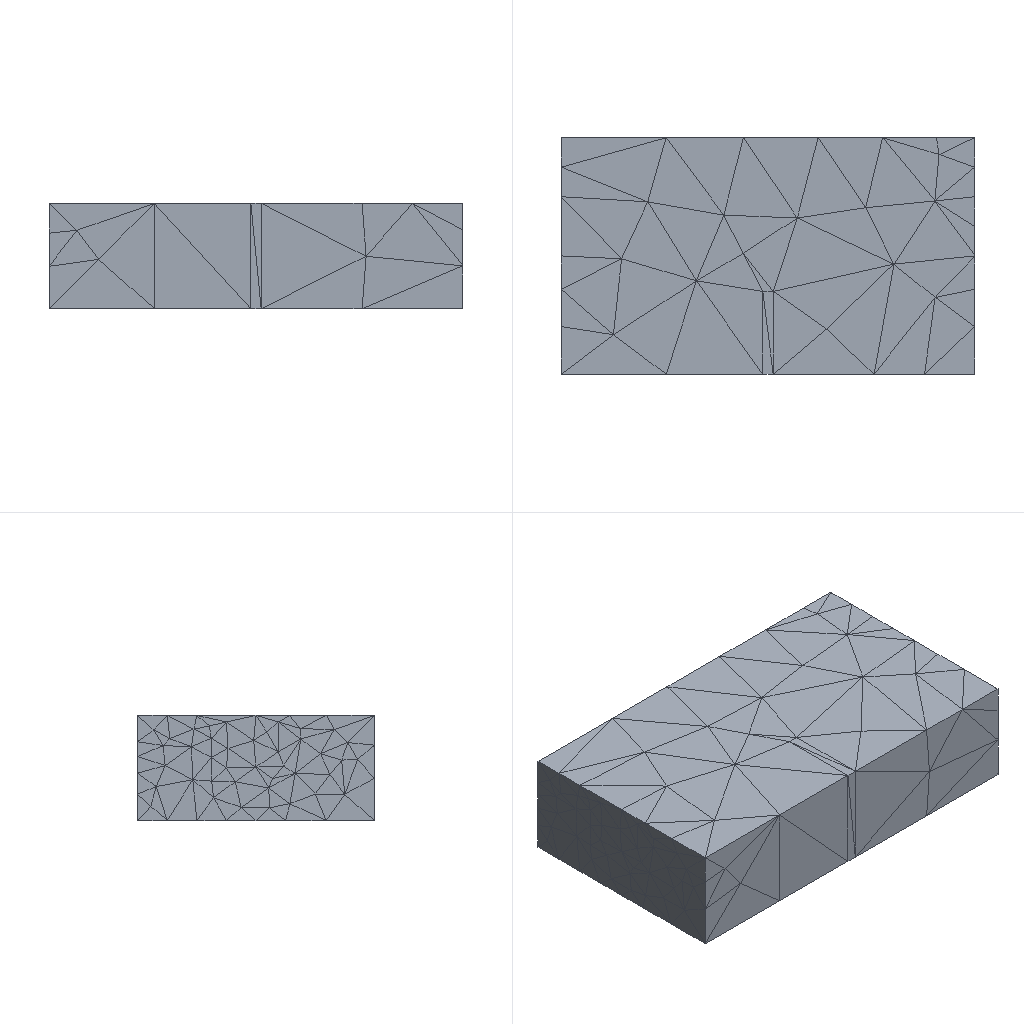Simulation study | ansys electronics desktop
Set-up summary:
category,name,step,type,value,unit,region
solver,ansys_electronics_desktop
units,length mm,,stated,model units
analysis,M16,,HFSS Modal Network,design_type=HFSS
setup,Setup1,M16,HfssDriven,frequency=10GHz; max_passes=2; max_delta_s=0.08
sweep,Sweep1,Setup1,Interpolating,8GHz..12GHz n=11 step=
mesh,nodes,,,n/a (no mesh stored)
mesh,elements,,,n/a (no mesh stored)
material,vacuum,,permittivity,1
load,P1,M16,wave port,,,objects 62
load,P2,M16,wave port,,,objects 74
bc,PerfE_VVAXO5,M16,perfect e,,,objects 86
bc,PerfE_TDHT5O,M16,perfect e,,,objects 98
bc,PerfE_5OTQQF,M16,perfect e,,,objects 110
bc,PerfE_AXHEQ4,M16,perfect e,,,objects 122
Ansys Electronics Desktop project file, long lists of numbers shortened, first 681 of 3558 lines:
$begin 'AnsoftProject'
	Created='Wed Sep 30 18:16:44 2026'
	Product='ElectronicsDesktop'
	FileOwnedByWorkbench=false
	$begin 'Desktop'
		Version(2026, 1)
		InfrastructureVersion(1, 0)
		$begin 'FactoryHeader'
			$begin 'geometry3deditor'
				KernelVersion(2, 0)
				ProjectContainsGeometry3D='1'
			$end 'geometry3deditor'
		$end 'FactoryHeader'
	$end 'Desktop'
	UsesAdvancedFeatures=false
	PreviewImageDesignId=1
	NextUniqueID=0
	MoveBackwards=false
	$begin 'HFSSEnvironment'
		Version(1, 0)
	$end 'HFSSEnvironment'
	$begin 'PlanarEMEnvironment'
		Version(1, 0)
	$end 'PlanarEMEnvironment'
	$begin 'Q3DEnvironment'
		Version(1, 0)
	$end 'Q3DEnvironment'
	$begin '2DExtractorEnvironment'
		Version(1, 0)
	$end '2DExtractorEnvironment'
	$begin 'NexximEnvironment'
		Version(1, 0)
	$end 'NexximEnvironment'
	$begin 'NexximNetlistEnvironment'
		Version(1, 0)
	$end 'NexximNetlistEnvironment'
	$begin 'EmitEnvironment'
		Version(1, 0)
	$end 'EmitEnvironment'
	$begin 'Maxwell3DEnvironment'
		Version(1, 0)
	$end 'Maxwell3DEnvironment'
	$begin 'Maxwell2DEnvironment'
		Version(1, 0)
	$end 'Maxwell2DEnvironment'
	$begin 'RMxprtEnvironment'
		Version(1, 0)
	$end 'RMxprtEnvironment'
	$begin 'MaxCirEnvironment'
		Version(1, 0)
	$end 'MaxCirEnvironment'
	$begin 'SimplorerEnvironment'
		Version(1, 0)
	$end 'SimplorerEnvironment'
	$begin 'IcepakEnvironment'
		Version(1, 0)
	$end 'IcepakEnvironment'
	$begin 'IcepakFEAEnvironment'
		Version(1, 0)
	$end 'IcepakFEAEnvironment'
	$begin 'SchematicEnvironment'
		Version(1, 0)
	$end 'SchematicEnvironment'
	$begin 'geometry3deditor'
		Version(1, 0)
	$end 'geometry3deditor'
	ReadVersion=12
	$begin 'DesignMgrEnvironment'
		CompInstCounter=1
		GPortCounter=0
		NetCounter=0
		Alias('Ieee;Simplorer Elements\\Ieee', 'Std;Simplorer Elements\\Std', 'Basic_VHDLAMS;Simplorer Elements\\Basic Elements VHDLAMS\\Basic Elements VHDLAMS', 'Digital_Elements;Simplorer Elements\\Digital Elements\\Digital Elements', 'Transformations;Simplorer Elements\\Tools\\Transformations\\Transformations', 'HEV_VHDLAMS;Simplorer Elements\\HEV VHDLAMS\\HEV VHDLAMS', 'automotive_vda;Simplorer Elem
	$end 'DesignMgrEnvironment'
	$begin 'ProjectDatasets'
		NextUniqueID=0
		MoveBackwards=false
		DatasetType='ProjectDatasetType'
		$begin 'DatasetDefinitions'
		$end 'DatasetDefinitions'
	$end 'ProjectDatasets'
	VariableOrders[0:]
	$begin 'Definitions'
		$begin 'Materials'
			$begin 'vacuum'
				CoordinateSystemType='Cartesian'
				BulkOrSurfaceType=1
				$begin 'PhysicsTypes'
					set('Electromagnetic')
				$end 'PhysicsTypes'
				$begin 'AttachedData'
					$begin 'MatAppearanceData'
						property_data='appearance_data'
						Red=230
						Green=230
						Blue=230
						Transparency=0.95
					$end 'MatAppearanceData'
				$end 'AttachedData'
				permittivity='1'
				ModTime=1499970477
				Library='Materials'
				LibLocation='SysLibrary'
				ModSinceLib=false
			$end 'vacuum'
		$end 'Materials'
		$begin 'SurfaceMaterials'
		$end 'SurfaceMaterials'
		$begin 'Scripts'
		$end 'Scripts'
		$begin 'AnsysComponents'
			NextUniqueID=0
			MoveBackwards=false
			$begin 'AnsysComponentDefinitions'
			$end 'AnsysComponentDefinitions'
		$end 'AnsysComponents'
		$begin 'Symbols'
			$begin 'M16'
				ModTime=1790763405
				Library=''
				ModSinceLib=false
				LibLocation='Project'
				HighestLevel=1
				Normalize=true
				InitialLevels(0, 1)
				$begin 'Graphics'
					Rect(0, 0, 0, 0, 0.00254, 0.00254, 0.00508, 0.00508, 0, 0, 0)
					Rect(0, 1, 0, 0, 0.0004233, 0.00254, 0.0004233, 0.0004233, 0, 0, 0)
				$end 'Graphics'
			$end 'M16'
		$end 'Symbols'
		$begin 'DefInfo'
			M16(1002, 0, 0, 0, '', 1790763405, '', 'M16', '', '', '', '', '', 'Design.bmp', '', 'Project', '', '', 1790763405, '', 0, 0)
		$end 'DefInfo'
		$begin 'Compdefs'
			$begin 'M16'
				Library=''
				CircuitEnv=0
				Refbase='U'
				NumParts=1
				ModSinceLib=true
				$begin 'Properties'
					TextProp('Representation', 'SRD', '', 'M16')
					TextProp('Owner', 'SRD', '', 'HFSS')
				$end 'Properties'
				CompExtID=6
				$begin 'Parameters'
					ButtonProp('CosimDefinition', 'D', '', 'Edit', 'Edit', 40501, ButtonPropClientData())
					MenuProp('CoSimulator', 'D', '', 'DefaultNetlist', 0)
				$end 'Parameters'
				$begin 'CosimDefinitions'
					$begin 'CosimDefinition'
						CosimulatorType=4
						CosimDefName='DefaultNetlist'
						IsDefinition=true
						Connect=true
						Data()
						GRef()
					$end 'CosimDefinition'
					DefaultCosim='DefaultNetlist'
				$end 'CosimDefinitions'
			$end 'M16'
		$end 'Compdefs'
	$end 'Definitions'
	DesignIDServer=2
	MoveBackwards=false
	$begin 'HFSSModel'
		RepRewriteV2=true
		Name='M16'
		DesignID=0
		'Use Advanced DC Extrapolation'=false
		'Use Power S'=false
		'Export FRTM After Simulation'=false
		'Export Rays After Simulation'=false
		'Export After Simulation'=false
		'Allow Material Override'=false
		'Calculate Lossy Dielectrics'=false
		'Perform Minimal validation'=false
		$begin 'TemperatureSettings'
			IncludeTemperatureDependence=false
			EnableFeedback=false
			Temperatures(6, '22cel', 34, '22cel', 62, '22cel', 74, '22cel', 86, '22cel', 98, '22cel', 110, '22cel', 122, '22cel')
		$end 'TemperatureSettings'
		ObjsEnabledForDeformation()
		'Port Validation Settings'='Standard'
		'Save Adaptive support files'=false
		SolutionType='HFSS Modal Network'
		$begin 'DrivenOptions'
			AutoOpen=false
		$end 'DrivenOptions'
		HasTransientSetups=false
		MaterialDensity=1
		MassOfTissue=1
		VoxelSize=1
		TissueObjectList=-1
		AverageSarMethod=0
		UseAutoDCThickness=true
		HaveZwaveSupport=true
		SolveInsideThreshold=100000
		RequireBodyFaceInfo=false
		$begin 'OutputVariable'
			NextUniqueID=0
			MoveBackwards=false
		$end 'OutputVariable'
		$begin 'ModelSetup'
			$begin 'DesignDatasets'
				NextUniqueID=0
				MoveBackwards=false
				DatasetType='DesignDatasetType'
				$begin 'DatasetDefinitions'
				$end 'DatasetDefinitions'
			$end 'DesignDatasets'
			VariableOrders[0:]
			$begin 'Editor3D Doc Preferences'
				BackgroundColorVersion=1
				'Plane Background'=0
				'Need Lights'=true
				'Ambient Light'=8355711
				'Num Lights'=1
				Light0[4: 16777215, 0.75, -0.15, -0.63]
				Ver=2
			$end 'Editor3D Doc Preferences'
			SnapMode=31
			WorkingCS=1
			$begin 'GeometryCore'
				BlockVersionID=3
				DataVersion=2
				NativeKernel='PARASOLID'
				NativeKernelVersionID=26
				Units='mm'
				ModelExtents=10000
				InstanceID=-1
				$begin 'ValidationOptions'
					EntityCheckLevel='Strict'
					IgnoreUnclassifiedObjects=false
					SkipIntersectionChecks=false
				$end 'ValidationOptions'
				ContainsGeomLinkUDM=false
				$begin 'GeometryOperations'
					BlockVersionID=2
					$begin 'AnsoftRangedIDServerManager'
						$begin 'AnsoftRangedIDServer'
							IDServerObjectTypeID=0
							IDServerRangeMin=0
							IDServerRangeMax=2146483647
							NextUniqueID=133
							MoveBackwards=false
						$end 'AnsoftRangedIDServer'
						$begin 'AnsoftRangedIDServer'
							IDServerObjectTypeID=1
							IDServerRangeMin=2146483648
							IDServerRangeMax=2146485547
							NextUniqueID=2146483654
							MoveBackwards=false
						$end 'AnsoftRangedIDServer'
					$end 'AnsoftRangedIDServerManager'
					StartBackGroundFaceID=2146483648
					$begin 'CoordinateSystems'
					$end 'CoordinateSystems'
					$begin 'OperandCSs'
					$end 'OperandCSs'
					$begin 'SubModelDefinitions'
					$end 'SubModelDefinitions'
					$begin 'Groups'
					$end 'Groups'
					$begin 'UserDefinedModels'
					$end 'UserDefinedModels'
					$begin 'OperandUserDefinedModels'
					$end 'OperandUserDefinedModels'
					$begin 'ToplevelParts'
						$begin 'GeometryPart'
							$begin 'Attributes'
								Name='WG'
								Flags=''
								Color='(230 230 230)'
								Transparency=0.8
								PartCoordinateSystem=1
								UDMId=-1
								GroupId=-1
								MaterialValue='"vacuum"'
								SurfaceMaterialValue='""'
								SolveInside=true
								ShellElement=false
								ShellElementThickness='0mm'
								ReferenceTemperature='20cel'
								IsMaterialEditable=true
								IsSurfaceMaterialEditable=true
								UseMaterialAppearance=false
								IsLightweight=false
								IsAlwaysHidden=false
							$end 'Attributes'
							$begin 'PhysicsAttributes'
								SuppressedForPhysics='False'
								SuppressedForPhysicsEditable=true
							$end 'PhysicsAttributes'
							$begin 'Operations'
								$begin 'Operation'
									OperationType='Box'
									ID=5
									ReferenceCoordSystemID=1
									$begin 'BoxParameters'
										KernelVersion=23
										XPosition='0mm'
										YPosition='0mm'
										ZPosition='0mm'
										XSize='40mm'
										YSize='22.86mm'
										ZSize='10.16mm'
									$end 'BoxParameters'
									ParentPartID=6
									ReferenceUDMID=-1
									IsSuppressed=false
									$begin 'OperationIdentity'
										$begin 'Topology'
											NumLumps=1
											NumShells=1
											NumFaces=6
											NumWires=0
											NumLoops=6
											NumCoedges=24
											NumEdges=12
											NumVertices=8
										$end 'Topology'
										BodyID=6
										StartFaceID=7
										StartEdgeID=13
										StartVertexID=25
										NumNewFaces=6
										NumNewEdges=12
										NumNewVertices=8
										FaceNameAndIDMap()
										EdgeNameAndIDMap()
										VertexNameAndIDMap()
									$end 'OperationIdentity'
								$end 'Operation'
							$end 'Operations'
							$begin 'SubregionDependencyInformation'
								ChildSubregions[0:]
							$end 'SubregionDependencyInformation'
						$end 'GeometryPart'
						$begin 'GeometryPart'
							$begin 'Attributes'
								Name='Iris'
								Flags=''
								Color='(230 230 230)'
								Transparency=0.8
								PartCoordinateSystem=1
								UDMId=-1
								GroupId=-1
								MaterialValue='"vacuum"'
								SurfaceMaterialValue='""'
								SolveInside=true
								ShellElement=false
								ShellElementThickness='0mm'
								ReferenceTemperature='20cel'
								IsMaterialEditable=true
								IsSurfaceMaterialEditable=true
								UseMaterialAppearance=false
								IsLightweight=false
								IsAlwaysHidden=false
							$end 'Attributes'
							$begin 'PhysicsAttributes'
								SuppressedForPhysics='False'
								SuppressedForPhysicsEditable=true
							$end 'PhysicsAttributes'
							$begin 'Operations'
								$begin 'Operation'
									OperationType='Box'
									ID=33
									ReferenceCoordSystemID=1
									$begin 'BoxParameters'
										KernelVersion=23
										XPosition='19.5mm'
										YPosition='0mm'
										ZPosition='0mm'
										XSize='1mm'
										YSize='8.001mm'
										ZSize='10.16mm'
									$end 'BoxParameters'
									ParentPartID=34
									ReferenceUDMID=-1
									IsSuppressed=false
									$begin 'OperationIdentity'
										$begin 'Topology'
											NumLumps=1
											NumShells=1
											NumFaces=6
											NumWires=0
											NumLoops=6
											NumCoedges=24
											NumEdges=12
											NumVertices=8
										$end 'Topology'
										BodyID=34
										StartFaceID=35
										StartEdgeID=41
										StartVertexID=53
										NumNewFaces=6
										NumNewEdges=12
										NumNewVertices=8
										FaceNameAndIDMap()
										EdgeNameAndIDMap()
										VertexNameAndIDMap()
									$end 'OperationIdentity'
								$end 'Operation'
							$end 'Operations'
							$begin 'SubregionDependencyInformation'
								ChildSubregions[0:]
							$end 'SubregionDependencyInformation'
						$end 'GeometryPart'
						$begin 'GeometryPart'
							$begin 'Attributes'
								Name='Port1'
								Flags=''
								Color='(230 230 230)'
								Transparency=0.8
								PartCoordinateSystem=1
								UDMId=-1
								GroupId=-1
								MaterialValue='"vacuum"'
								SurfaceMaterialValue='""'
								SolveInside=true
								ShellElement=false
								ShellElementThickness='0mm'
								ReferenceTemperature='20cel'
								IsMaterialEditable=true
								IsSurfaceMaterialEditable=true
								UseMaterialAppearance=false
								IsLightweight=false
								IsAlwaysHidden=false
							$end 'Attributes'
							$begin 'PhysicsAttributes'
								SuppressedForPhysics='False'
								SuppressedForPhysicsEditable=true
							$end 'PhysicsAttributes'
							$begin 'Operations'
								$begin 'Operation'
									OperationType='Rectangle'
									ID=61
									ReferenceCoordSystemID=1
									$begin 'RectangleParameters'
										KernelVersion=23
										XStart='0mm'
										YStart='0mm'
										ZStart='0mm'
										Width='22.86mm'
										Height='10.16mm'
										WhichAxis='X'
									$end 'RectangleParameters'
									ParentPartID=62
									ReferenceUDMID=-1
									IsSuppressed=false
									$begin 'OperationIdentity'
										$begin 'Topology'
											NumLumps=1
											NumShells=1
											NumFaces=0
											NumWires=1
											NumLoops=0
											NumCoedges=0
											NumEdges=4
											NumVertices=4
										$end 'Topology'
										BodyID=62
										StartFaceID=-1
										StartEdgeID=63
										StartVertexID=67
										NumNewFaces=0
										NumNewEdges=4
										NumNewVertices=4
										FaceNameAndIDMap()
										EdgeNameAndIDMap()
										VertexNameAndIDMap()
									$end 'OperationIdentity'
								$end 'Operation'
								$begin 'Operation'
									OperationType='CoverLines'
									ID=71
									$begin 'LocalOperationParameters'
										KernelVersion=23
										LocalOpPart=62
									$end 'LocalOperationParameters'
									ParentPartID=62
									ReferenceUDMID=-1
									IsSuppressed=false
									$begin 'OperationIdentity'
										$begin 'Topology'
											NumLumps=1
											NumShells=1
											NumFaces=1
											NumWires=0
											NumLoops=1
											NumCoedges=4
											NumEdges=4
											NumVertices=4
										$end 'Topology'
										BodyID=-1
										StartFaceID=72
										StartEdgeID=-1
										StartVertexID=-1
										NumNewFaces=1
										NumNewEdges=0
										NumNewVertices=0
										FaceNameAndIDMap()
										EdgeNameAndIDMap()
										VertexNameAndIDMap()
										$begin 'GeomTopolBasedOperationIdentityHelper'
											$begin 'NewFaces'
												$begin 'Face'
													NormalizedSerialNum=0
													ID=72
													$begin 'FaceGeomTopol'
														FaceTopol(1, 4, 4, 4)
														$begin 'FaceGeometry'
															Area=232.258
															FcUVMid(1.51681195174844e-15, 11.43, 5.08)
															$begin 'FcTolVts'
																TolVt(0, 0, 0, 5e-07)
																TolVt(1.39977129142543e-15, 22.86, 5.07593966858622e-15, 5e-07)
																TolVt(3.03362390349689e-15, 22.86, 10.16, 5e-07)
																TolVt(1.63385261207146e-15, -2.25597318603832e-15, 10.16, 5e-07)
															$end 'FcTolVts'
														$end 'FaceGeometry'
													$end 'FaceGeomTopol'
												$end 'Face'
											$end 'NewFaces'
											$begin 'NewEdges'
											$end 'NewEdges'
											$begin 'NewVertices'
											$end 'NewVertices'
										$end 'GeomTopolBasedOperationIdentityHelper'
									$end 'OperationIdentity'
									ParentOperationID=61
								$end 'Operation'
							$end 'Operations'
							$begin 'SubregionDependencyInformation'
								ChildSubregions[0:]
							$end 'SubregionDependencyInformation'
						$end 'GeometryPart'
						$begin 'GeometryPart'
							$begin 'Attributes'
								Name='Port2'
								Flags=''
								Color='(230 230 230)'
								Transparency=0.8
								PartCoordinateSystem=1
								UDMId=-1
								GroupId=-1
								MaterialValue='"vacuum"'
								SurfaceMaterialValue='""'
								SolveInside=true
								ShellElement=false
								ShellElementThickness='0mm'
								ReferenceTemperature='20cel'
								IsMaterialEditable=true
								IsSurfaceMaterialEditable=true
								UseMaterialAppearance=false
								IsLightweight=false
								IsAlwaysHidden=false
							$end 'Attributes'
							$begin 'PhysicsAttributes'
								SuppressedForPhysics='False'
								SuppressedForPhysicsEditable=true
							$end 'PhysicsAttributes'
							$begin 'Operations'
								$begin 'Operation'
									OperationType='Rectangle'
									ID=73
									ReferenceCoordSystemID=1
									$begin 'RectangleParameters'
										KernelVersion=23
										XStart='40mm'
										YStart='0mm'
										ZStart='0mm'
										Width='22.86mm'
										Height='10.16mm'
										WhichAxis='X'
									$end 'RectangleParameters'
									ParentPartID=74
									ReferenceUDMID=-1
									IsSuppressed=false
									$begin 'OperationIdentity'
										$begin 'Topology'
											NumLumps=1
											NumShells=1
											NumFaces=0
											NumWires=1
											NumLoops=0
											NumCoedges=0
											NumEdges=4
											NumVertices=4
										$end 'Topology'
										BodyID=74
										StartFaceID=-1
										StartEdgeID=75
										StartVertexID=79
										NumNewFaces=0
										NumNewEdges=4
										NumNewVertices=4
										FaceNameAndIDMap()
										EdgeNameAndIDMap()
										VertexNameAndIDMap()
									$end 'OperationIdentity'
								$end 'Operation'
								$begin 'Operation'
									OperationType='CoverLines'
									ID=83
									$begin 'LocalOperationParameters'
										KernelVersion=23
										LocalOpPart=74
									$end 'LocalOperationParameters'
									ParentPartID=74
									ReferenceUDMID=-1
									IsSuppressed=false
									$begin 'OperationIdentity'
										$begin 'Topology'
											NumLumps=1
											NumShells=1
											NumFaces=1
											NumWires=0
											NumLoops=1
											NumCoedges=4
											NumEdges=4
											NumVertices=4
										$end 'Topology'
										BodyID=-1
										StartFaceID=84
										StartEdgeID=-1
										StartVertexID=-1
										NumNewFaces=1
										NumNewEdges=0
										NumNewVertices=0
										FaceNameAndIDMap()
										EdgeNameAndIDMap()
										VertexNameAndIDMap()
										$begin 'GeomTopolBasedOperationIdentityHelper'
											$begin 'NewFaces'
												$begin 'Face'
													NormalizedSerialNum=0
													ID=84
													$begin 'FaceGeomTopol'
														FaceTopol(1, 4, 4, 4)
														$begin 'FaceGeometry'
															Area=232.258
															FcUVMid(40, 11.43, 5.08)
															$begin 'FcTolVts'
																TolVt(40, 0, 0, 5e-07)
																TolVt(40, 22.86, 5.07593966858622e-15, 5e-07)
																TolVt(40, 22.86, 10.16, 5e-07)
																TolVt(40, -2.25597318603832e-15, 10.16, 5e-07)
															$end 'FcTolVts'
														$end 'FaceGeometry'
													$end 'FaceGeomTopol'
												$end 'Face'
											$end 'NewFaces'
											$begin 'NewEdges'
											$end 'NewEdges'
											$begin 'NewVertices'
											$end 'NewVertices'
										$end 'GeomTopolBasedOperationIdentityHelper'
									$end 'OperationIdentity'
									ParentOperationID=73
								$end 'Operation'
							$end 'Operations'
							$begin 'SubregionDependencyInformation'
								ChildSubregions[0:]
							$end 'SubregionDependencyInformation'
						$end 'GeometryPart'
						$begin 'GeometryPart'
							$begin 'Attributes'
								Name='W0'
								Flags=''
								Color='(230 230 230)'
								Transparency=0.8
								PartCoordinateSystem=1
								UDMId=-1
								GroupId=-1
								MaterialValue='"vacuum"'
								SurfaceMaterialValue='""'
								SolveInside=true
								ShellElement=false
								ShellElementThickness='0mm'
Last 1296 lines:
														AxisScale='Linear'
														NumberFormat='Auto'
														$begin 'TextFont'
															$begin 'FontAttribute'
																$begin 'Font'
																	HeightInPts=9
																	Width=0
																	Escapement=0
																	Orientation=0
																	Weight=400
																	Italic=0
																	Underline=0
																	StrikeOut=0
																	CharSet=0
																	OutPrecision=7
																	ClipPrecision=48
																	Quality=6
																	PitchAndFamily=0
																	FaceName='Arial'
																$end 'Font'
																ColorVersion=1
															$end 'FontAttribute'
														$end 'TextFont'
														InfMapMode=false
														InfMapValue=1.79769313486232e+306
														AutoRangeMin=true
														AutoRangeMax=true
														AutoSpacing=true
														kNumMinorDivisions=5
														ShowAxisTitle=true
														ShowAxisUnits=true
														vwm='FullWnd'
														viewWndWd=#nan
														ActivateMargins=true
														MarginPercent=0
														NeverCollapse=false
														AxisStripes=true
													$end 'LineAxisRenderAttribute'
												$end 'SubMapItem'
												$begin 'SubMapItem'
													DataSourceID=2
													$begin 'LineAxisRenderAttribute'
														DecimalFieldWidth=3
														DecimalFieldPrecision=2
														ManualTitle=''
														ColorVersion=1
														MinScale=0
														MaxScale=1
														TickSpacing=1
														ManualUnits=false
														Units='mm'
														AxisScale='Linear'
														NumberFormat='Auto'
														$begin 'TextFont'
															$begin 'FontAttribute'
																$begin 'Font'
																	HeightInPts=9
																	Width=0
																	Escapement=0
																	Orientation=0
																	Weight=400
																	Italic=0
																	Underline=0
																	StrikeOut=0
																	CharSet=0
																	OutPrecision=7
																	ClipPrecision=48
																	Quality=6
																	PitchAndFamily=0
																	FaceName='Arial'
																$end 'Font'
																ColorVersion=1
															$end 'FontAttribute'
														$end 'TextFont'
														InfMapMode=false
														InfMapValue=1.79769313486232e+306
														AutoRangeMin=true
														AutoRangeMax=true
														AutoSpacing=true
														kNumMinorDivisions=5
														ShowAxisTitle=true
														ShowAxisUnits=true
														vwm='FullWnd'
														viewWndWd=#nan
														ActivateMargins=true
														MarginPercent=0
														NeverCollapse=false
														AxisStripes=true
													$end 'LineAxisRenderAttribute'
												$end 'SubMapItem'
												$begin 'SubMapItem'
													DataSourceID=8
													$begin 'LineAxisRenderAttribute'
														DecimalFieldWidth=3
														DecimalFieldPrecision=2
														ManualTitle=''
														ColorVersion=1
														MinScale=0
														MaxScale=1
														TickSpacing=1
														ManualUnits=false
														Units='mm'
														AxisScale='Linear'
														NumberFormat='Auto'
														$begin 'TextFont'
															$begin 'FontAttribute'
																$begin 'Font'
																	HeightInPts=9
																	Width=0
																	Escapement=0
																	Orientation=0
																	Weight=400
																	Italic=0
																	Underline=0
																	StrikeOut=0
																	CharSet=0
																	OutPrecision=7
																	ClipPrecision=48
																	Quality=6
																	PitchAndFamily=0
																	FaceName='Arial'
																$end 'Font'
																ColorVersion=1
															$end 'FontAttribute'
														$end 'TextFont'
														InfMapMode=false
														InfMapValue=1.79769313486232e+306
														AutoRangeMin=true
														AutoRangeMax=true
														AutoSpacing=true
														kNumMinorDivisions=5
														ShowAxisTitle=true
														ShowAxisUnits=true
														vwm='FullWnd'
														viewWndWd=#nan
														ActivateMargins=true
														MarginPercent=0
														NeverCollapse=false
														AxisStripes=true
													$end 'LineAxisRenderAttribute'
												$end 'SubMapItem'
												$begin 'SubMapItem'
													DataSourceID=9
													$begin 'LineAxisRenderAttribute'
														DecimalFieldWidth=3
														DecimalFieldPrecision=2
														ManualTitle=''
														ColorVersion=1
														MinScale=0
														MaxScale=1
														TickSpacing=1
														ManualUnits=false
														Units='mm'
														AxisScale='Linear'
														NumberFormat='Auto'
														$begin 'TextFont'
															$begin 'FontAttribute'
																$begin 'Font'
																	HeightInPts=9
																	Width=0
																	Escapement=0
																	Orientation=0
																	Weight=400
																	Italic=0
																	Underline=0
																	StrikeOut=0
																	CharSet=0
																	OutPrecision=7
																	ClipPrecision=48
																	Quality=6
																	PitchAndFamily=0
																	FaceName='Arial'
																$end 'Font'
																ColorVersion=1
															$end 'FontAttribute'
														$end 'TextFont'
														InfMapMode=false
														InfMapValue=1.79769313486232e+306
														AutoRangeMin=true
														AutoRangeMax=true
														AutoSpacing=true
														kNumMinorDivisions=5
														ShowAxisTitle=true
														ShowAxisUnits=true
														vwm='FullWnd'
														viewWndWd=#nan
														ActivateMargins=true
														MarginPercent=0
														NeverCollapse=false
														AxisStripes=true
													$end 'LineAxisRenderAttribute'
												$end 'SubMapItem'
												$begin 'SubMapItem'
													DataSourceID=10
													$begin 'LineAxisRenderAttribute'
														DecimalFieldWidth=3
														DecimalFieldPrecision=2
														ManualTitle=''
														ColorVersion=1
														MinScale=0
														MaxScale=1
														TickSpacing=1
														ManualUnits=false
														Units='mm'
														AxisScale='Linear'
														NumberFormat='Auto'
														$begin 'TextFont'
															$begin 'FontAttribute'
																$begin 'Font'
																	HeightInPts=9
																	Width=0
																	Escapement=0
																	Orientation=0
																	Weight=400
																	Italic=0
																	Underline=0
																	StrikeOut=0
																	CharSet=0
																	OutPrecision=7
																	ClipPrecision=48
																	Quality=6
																	PitchAndFamily=0
																	FaceName='Arial'
																$end 'Font'
																ColorVersion=1
															$end 'FontAttribute'
														$end 'TextFont'
														InfMapMode=false
														InfMapValue=1.79769313486232e+306
														AutoRangeMin=true
														AutoRangeMax=true
														AutoSpacing=true
														kNumMinorDivisions=5
														ShowAxisTitle=true
														ShowAxisUnits=true
														vwm='FullWnd'
														viewWndWd=#nan
														ActivateMargins=true
														MarginPercent=0
														NeverCollapse=false
														AxisStripes=true
													$end 'LineAxisRenderAttribute'
												$end 'SubMapItem'
												$begin 'SubMapItem'
													DataSourceID=11
													$begin 'LineAxisRenderAttribute'
														DecimalFieldWidth=3
														DecimalFieldPrecision=2
														ManualTitle=''
														ColorVersion=1
														MinScale=0
														MaxScale=1
														TickSpacing=1
														ManualUnits=false
														Units='mm'
														AxisScale='Linear'
														NumberFormat='Auto'
														$begin 'TextFont'
															$begin 'FontAttribute'
																$begin 'Font'
																	HeightInPts=9
																	Width=0
																	Escapement=0
																	Orientation=0
																	Weight=400
																	Italic=0
																	Underline=0
																	StrikeOut=0
																	CharSet=0
																	OutPrecision=7
																	ClipPrecision=48
																	Quality=6
																	PitchAndFamily=0
																	FaceName='Arial'
																$end 'Font'
																ColorVersion=1
															$end 'FontAttribute'
														$end 'TextFont'
														InfMapMode=false
														InfMapValue=1.79769313486232e+306
														AutoRangeMin=true
														AutoRangeMax=true
														AutoSpacing=true
														kNumMinorDivisions=5
														ShowAxisTitle=true
														ShowAxisUnits=true
														vwm='FullWnd'
														viewWndWd=#nan
														ActivateMargins=true
														MarginPercent=0
														NeverCollapse=false
														AxisStripes=true
													$end 'LineAxisRenderAttribute'
												$end 'SubMapItem'
												$begin 'SubMapItem'
													DataSourceID=12
													$begin 'LineAxisRenderAttribute'
														DecimalFieldWidth=3
														DecimalFieldPrecision=2
														ManualTitle=''
														ColorVersion=1
														MinScale=0
														MaxScale=1
														TickSpacing=1
														ManualUnits=false
														Units='mm'
														AxisScale='Linear'
														NumberFormat='Auto'
														$begin 'TextFont'
															$begin 'FontAttribute'
																$begin 'Font'
																	HeightInPts=9
																	Width=0
																	Escapement=0
																	Orientation=0
																	Weight=400
																	Italic=0
																	Underline=0
																	StrikeOut=0
																	CharSet=0
																	OutPrecision=7
																	ClipPrecision=48
																	Quality=6
																	PitchAndFamily=0
																	FaceName='Arial'
																$end 'Font'
																ColorVersion=1
															$end 'FontAttribute'
														$end 'TextFont'
														InfMapMode=false
														InfMapValue=1.79769313486232e+306
														AutoRangeMin=true
														AutoRangeMax=true
														AutoSpacing=true
														kNumMinorDivisions=5
														ShowAxisTitle=true
														ShowAxisUnits=true
														vwm='FullWnd'
														viewWndWd=#nan
														ActivateMargins=true
														MarginPercent=0
														NeverCollapse=false
														AxisStripes=true
													$end 'LineAxisRenderAttribute'
												$end 'SubMapItem'
												$begin 'SubMapItem'
													DataSourceID=13
													$begin 'LineAxisRenderAttribute'
														DecimalFieldWidth=3
														DecimalFieldPrecision=2
														ManualTitle=''
														ColorVersion=1
														MinScale=0
														MaxScale=1
														TickSpacing=1
														ManualUnits=false
														Units='mm'
														AxisScale='Linear'
														NumberFormat='Auto'
														$begin 'TextFont'
															$begin 'FontAttribute'
																$begin 'Font'
																	HeightInPts=9
																	Width=0
																	Escapement=0
																	Orientation=0
																	Weight=400
																	Italic=0
																	Underline=0
																	StrikeOut=0
																	CharSet=0
																	OutPrecision=7
																	ClipPrecision=48
																	Quality=6
																	PitchAndFamily=0
																	FaceName='Arial'
																$end 'Font'
																ColorVersion=1
															$end 'FontAttribute'
														$end 'TextFont'
														InfMapMode=false
														InfMapValue=1.79769313486232e+306
														AutoRangeMin=true
														AutoRangeMax=true
														AutoSpacing=true
														kNumMinorDivisions=5
														ShowAxisTitle=true
														ShowAxisUnits=true
														vwm='FullWnd'
														viewWndWd=#nan
														ActivateMargins=true
														MarginPercent=0
														NeverCollapse=false
														AxisStripes=true
													$end 'LineAxisRenderAttribute'
												$end 'SubMapItem'
												$begin 'SubMapItem'
													DataSourceID=14
													$begin 'LineAxisRenderAttribute'
														DecimalFieldWidth=3
														DecimalFieldPrecision=2
														ManualTitle=''
														ColorVersion=1
														MinScale=0
														MaxScale=1
														TickSpacing=1
														ManualUnits=false
														Units='mm'
														AxisScale='Linear'
														NumberFormat='Auto'
														$begin 'TextFont'
															$begin 'FontAttribute'
																$begin 'Font'
																	HeightInPts=9
																	Width=0
																	Escapement=0
																	Orientation=0
																	Weight=400
																	Italic=0
																	Underline=0
																	StrikeOut=0
																	CharSet=0
																	OutPrecision=7
																	ClipPrecision=48
																	Quality=6
																	PitchAndFamily=0
																	FaceName='Arial'
																$end 'Font'
																ColorVersion=1
															$end 'FontAttribute'
														$end 'TextFont'
														InfMapMode=false
														InfMapValue=1.79769313486232e+306
														AutoRangeMin=true
														AutoRangeMax=true
														AutoSpacing=true
														kNumMinorDivisions=5
														ShowAxisTitle=true
														ShowAxisUnits=true
														vwm='FullWnd'
														viewWndWd=#nan
														ActivateMargins=true
														MarginPercent=0
														NeverCollapse=false
														AxisStripes=true
													$end 'LineAxisRenderAttribute'
												$end 'SubMapItem'
												$begin 'SubMapItem'
													DataSourceID=15
													$begin 'LineAxisRenderAttribute'
														DecimalFieldWidth=3
														DecimalFieldPrecision=2
														ManualTitle=''
														ColorVersion=1
														MinScale=0
														MaxScale=1
														TickSpacing=1
														ManualUnits=false
														Units='mm'
														AxisScale='Linear'
														NumberFormat='Auto'
														$begin 'TextFont'
															$begin 'FontAttribute'
																$begin 'Font'
																	HeightInPts=9
																	Width=0
																	Escapement=0
																	Orientation=0
																	Weight=400
																	Italic=0
																	Underline=0
																	StrikeOut=0
																	CharSet=0
																	OutPrecision=7
																	ClipPrecision=48
																	Quality=6
																	PitchAndFamily=0
																	FaceName='Arial'
																$end 'Font'
																ColorVersion=1
															$end 'FontAttribute'
														$end 'TextFont'
														InfMapMode=false
														InfMapValue=1.79769313486232e+306
														AutoRangeMin=true
														AutoRangeMax=true
														AutoSpacing=true
														kNumMinorDivisions=5
														ShowAxisTitle=true
														ShowAxisUnits=true
														vwm='FullWnd'
														viewWndWd=#nan
														ActivateMargins=true
														MarginPercent=0
														NeverCollapse=false
														AxisStripes=true
													$end 'LineAxisRenderAttribute'
												$end 'SubMapItem'
												$begin 'SubMapItem'
													DataSourceID=16
													$begin 'LineAxisRenderAttribute'
														DecimalFieldWidth=3
														DecimalFieldPrecision=2
														ManualTitle=''
														ColorVersion=1
														MinScale=0
														MaxScale=1
														TickSpacing=1
														ManualUnits=false
														Units='mm'
														AxisScale='Linear'
														NumberFormat='Auto'
														$begin 'TextFont'
															$begin 'FontAttribute'
																$begin 'Font'
																	HeightInPts=9
																	Width=0
																	Escapement=0
																	Orientation=0
																	Weight=400
																	Italic=0
																	Underline=0
																	StrikeOut=0
																	CharSet=0
																	OutPrecision=7
																	ClipPrecision=48
																	Quality=6
																	PitchAndFamily=0
																	FaceName='Arial'
																$end 'Font'
																ColorVersion=1
															$end 'FontAttribute'
														$end 'TextFont'
														InfMapMode=false
														InfMapValue=1.79769313486232e+306
														AutoRangeMin=true
														AutoRangeMax=true
														AutoSpacing=true
														kNumMinorDivisions=5
														ShowAxisTitle=true
														ShowAxisUnits=true
														vwm='FullWnd'
														viewWndWd=#nan
														ActivateMargins=true
														MarginPercent=0
														NeverCollapse=false
														AxisStripes=true
													$end 'LineAxisRenderAttribute'
												$end 'SubMapItem'
												$begin 'SubMapItem'
													DataSourceID=17
													$begin 'LineAxisRenderAttribute'
														DecimalFieldWidth=3
														DecimalFieldPrecision=2
														ManualTitle=''
														ColorVersion=1
														MinScale=0
														MaxScale=1
														TickSpacing=1
														ManualUnits=false
														Units='mm'
														AxisScale='Linear'
														NumberFormat='Auto'
														$begin 'TextFont'
															$begin 'FontAttribute'
																$begin 'Font'
																	HeightInPts=9
																	Width=0
																	Escapement=0
																	Orientation=0
																	Weight=400
																	Italic=0
																	Underline=0
																	StrikeOut=0
																	CharSet=0
																	OutPrecision=7
																	ClipPrecision=48
																	Quality=6
																	PitchAndFamily=0
																	FaceName='Arial'
																$end 'Font'
																ColorVersion=1
															$end 'FontAttribute'
														$end 'TextFont'
														InfMapMode=false
														InfMapValue=1.79769313486232e+306
														AutoRangeMin=true
														AutoRangeMax=true
														AutoSpacing=true
														kNumMinorDivisions=5
														ShowAxisTitle=true
														ShowAxisUnits=true
														vwm='FullWnd'
														viewWndWd=#nan
														ActivateMargins=true
														MarginPercent=0
														NeverCollapse=false
														AxisStripes=true
													$end 'LineAxisRenderAttribute'
												$end 'SubMapItem'
												$begin 'SubMapItem'
													DataSourceID=18
													$begin 'LineAxisRenderAttribute'
														DecimalFieldWidth=3
														DecimalFieldPrecision=2
														ManualTitle=''
														ColorVersion=1
														MinScale=0
														MaxScale=1
														TickSpacing=1
														ManualUnits=false
														Units='mm'
														AxisScale='Linear'
														NumberFormat='Auto'
														$begin 'TextFont'
															$begin 'FontAttribute'
																$begin 'Font'
																	HeightInPts=9
																	Width=0
																	Escapement=0
																	Orientation=0
																	Weight=400
																	Italic=0
																	Underline=0
																	StrikeOut=0
																	CharSet=0
																	OutPrecision=7
																	ClipPrecision=48
																	Quality=6
																	PitchAndFamily=0
																	FaceName='Arial'
																$end 'Font'
																ColorVersion=1
															$end 'FontAttribute'
														$end 'TextFont'
														InfMapMode=false
														InfMapValue=1.79769313486232e+306
														AutoRangeMin=true
														AutoRangeMax=true
														AutoSpacing=true
														kNumMinorDivisions=5
														ShowAxisTitle=true
														ShowAxisUnits=true
														vwm='FullWnd'
														viewWndWd=#nan
														ActivateMargins=true
														MarginPercent=0
														NeverCollapse=false
														AxisStripes=true
													$end 'LineAxisRenderAttribute'
												$end 'SubMapItem'
												$begin 'SubMapItem'
													DataSourceID=19
													$begin 'LineAxisRenderAttribute'
														DecimalFieldWidth=3
														DecimalFieldPrecision=2
														ManualTitle=''
														ColorVersion=1
														MinScale=0
														MaxScale=1
														TickSpacing=1
														ManualUnits=false
														Units='mm'
														AxisScale='Linear'
														NumberFormat='Auto'
														$begin 'TextFont'
															$begin 'FontAttribute'
																$begin 'Font'
																	HeightInPts=9
																	Width=0
																	Escapement=0
																	Orientation=0
																	Weight=400
																	Italic=0
																	Underline=0
																	StrikeOut=0
																	CharSet=0
																	OutPrecision=7
																	ClipPrecision=48
																	Quality=6
																	PitchAndFamily=0
																	FaceName='Arial'
																$end 'Font'
																ColorVersion=1
															$end 'FontAttribute'
														$end 'TextFont'
														InfMapMode=false
														InfMapValue=1.79769313486232e+306
														AutoRangeMin=true
														AutoRangeMax=true
														AutoSpacing=true
														kNumMinorDivisions=5
														ShowAxisTitle=true
														ShowAxisUnits=true
														vwm='FullWnd'
														viewWndWd=#nan
														ActivateMargins=true
														MarginPercent=0
														NeverCollapse=false
														AxisStripes=true
													$end 'LineAxisRenderAttribute'
												$end 'SubMapItem'
												$begin 'SubMapItem'
													DataSourceID=20
													$begin 'LineAxisRenderAttribute'
														DecimalFieldWidth=3
														DecimalFieldPrecision=2
														ManualTitle=''
														ColorVersion=1
														MinScale=0
														MaxScale=1
														TickSpacing=1
														ManualUnits=false
														Units='mm'
														AxisScale='Linear'
														NumberFormat='Auto'
														$begin 'TextFont'
															$begin 'FontAttribute'
																$begin 'Font'
																	HeightInPts=9
																	Width=0
																	Escapement=0
																	Orientation=0
																	Weight=400
																	Italic=0
																	Underline=0
																	StrikeOut=0
																	CharSet=0
																	OutPrecision=7
																	ClipPrecision=48
																	Quality=6
																	PitchAndFamily=0
																	FaceName='Arial'
																$end 'Font'
																ColorVersion=1
															$end 'FontAttribute'
														$end 'TextFont'
														InfMapMode=false
														InfMapValue=1.79769313486232e+306
														AutoRangeMin=true
														AutoRangeMax=true
														AutoSpacing=true
														kNumMinorDivisions=5
														ShowAxisTitle=true
														ShowAxisUnits=true
														vwm='FullWnd'
														viewWndWd=#nan
														ActivateMargins=true
														MarginPercent=0
														NeverCollapse=false
														AxisStripes=true
													$end 'LineAxisRenderAttribute'
												$end 'SubMapItem'
												$begin 'SubMapItem'
													DataSourceID=21
													$begin 'LineAxisRenderAttribute'
														DecimalFieldWidth=3
														DecimalFieldPrecision=2
														ManualTitle=''
														ColorVersion=1
														MinScale=0
														MaxScale=1
														TickSpacing=1
														ManualUnits=false
														Units='mm'
														AxisScale='Linear'
														NumberFormat='Auto'
														$begin 'TextFont'
															$begin 'FontAttribute'
																$begin 'Font'
																	HeightInPts=9
																	Width=0
																	Escapement=0
																	Orientation=0
																	Weight=400
																	Italic=0
																	Underline=0
																	StrikeOut=0
																	CharSet=0
																	OutPrecision=7
																	ClipPrecision=48
																	Quality=6
																	PitchAndFamily=0
																	FaceName='Arial'
																$end 'Font'
																ColorVersion=1
															$end 'FontAttribute'
														$end 'TextFont'
														InfMapMode=false
														InfMapValue=1.79769313486232e+306
														AutoRangeMin=true
														AutoRangeMax=true
														AutoSpacing=true
														kNumMinorDivisions=5
														ShowAxisTitle=true
														ShowAxisUnits=true
														vwm='FullWnd'
														viewWndWd=#nan
														ActivateMargins=true
														MarginPercent=0
														NeverCollapse=false
														AxisStripes=true
													$end 'LineAxisRenderAttribute'
												$end 'SubMapItem'
												$begin 'SubMapItem'
													DataSourceID=22
													$begin 'LineAxisRenderAttribute'
														DecimalFieldWidth=3
														DecimalFieldPrecision=2
														ManualTitle=''
														ColorVersion=1
														MinScale=0
														MaxScale=1
														TickSpacing=1
														ManualUnits=false
														Units='mm'
														AxisScale='Linear'
														NumberFormat='Auto'
														$begin 'TextFont'
															$begin 'FontAttribute'
																$begin 'Font'
																	HeightInPts=9
																	Width=0
																	Escapement=0
																	Orientation=0
																	Weight=400
																	Italic=0
																	Underline=0
																	StrikeOut=0
																	CharSet=0
																	OutPrecision=7
																	ClipPrecision=48
																	Quality=6
																	PitchAndFamily=0
																	FaceName='Arial'
																$end 'Font'
																ColorVersion=1
															$end 'FontAttribute'
														$end 'TextFont'
														InfMapMode=false
														InfMapValue=1.79769313486232e+306
														AutoRangeMin=true
														AutoRangeMax=true
														AutoSpacing=true
														kNumMinorDivisions=5
														ShowAxisTitle=true
														ShowAxisUnits=true
														vwm='FullWnd'
														viewWndWd=#nan
														ActivateMargins=true
														MarginPercent=0
														NeverCollapse=false
														AxisStripes=true
													$end 'LineAxisRenderAttribute'
												$end 'SubMapItem'
												$begin 'SubMapItem'
													DataSourceID=23
													$begin 'LineAxisRenderAttribute'
														DecimalFieldWidth=3
														DecimalFieldPrecision=2
														ManualTitle=''
														ColorVersion=1
														MinScale=0
														MaxScale=1
														TickSpacing=1
														ManualUnits=false
														Units='mm'
														AxisScale='Linear'
														NumberFormat='Auto'
														$begin 'TextFont'
															$begin 'FontAttribute'
																$begin 'Font'
																	HeightInPts=9
																	Width=0
																	Escapement=0
																	Orientation=0
																	Weight=400
																	Italic=0
																	Underline=0
																	StrikeOut=0
																	CharSet=0
																	OutPrecision=7
																	ClipPrecision=48
																	Quality=6
																	PitchAndFamily=0
																	FaceName='Arial'
																$end 'Font'
																ColorVersion=1
															$end 'FontAttribute'
														$end 'TextFont'
														InfMapMode=false
														InfMapValue=1.79769313486232e+306
														AutoRangeMin=true
														AutoRangeMax=true
														AutoSpacing=true
														kNumMinorDivisions=5
														ShowAxisTitle=true
														ShowAxisUnits=true
														vwm='FullWnd'
														viewWndWd=#nan
														ActivateMargins=true
														MarginPercent=0
														NeverCollapse=false
														AxisStripes=true
													$end 'LineAxisRenderAttribute'
												$end 'SubMapItem'
												$begin 'SubMapItem'
													DataSourceID=24
													$begin 'LineAxisRenderAttribute'
														DecimalFieldWidth=3
														DecimalFieldPrecision=2
														ManualTitle=''
														ColorVersion=1
														MinScale=0
														MaxScale=1
														TickSpacing=1
														ManualUnits=false
														Units='mm'
														AxisScale='Linear'
														NumberFormat='Auto'
														$begin 'TextFont'
															$begin 'FontAttribute'
																$begin 'Font'
																	HeightInPts=9
																	Width=0
																	Escapement=0
																	Orientation=0
																	Weight=400
																	Italic=0
																	Underline=0
																	StrikeOut=0
																	CharSet=0
																	OutPrecision=7
																	ClipPrecision=48
																	Quality=6
																	PitchAndFamily=0
																	FaceName='Arial'
																$end 'Font'
																ColorVersion=1
															$end 'FontAttribute'
														$end 'TextFont'
														InfMapMode=false
														InfMapValue=1.79769313486232e+306
														AutoRangeMin=true
														AutoRangeMax=true
														AutoSpacing=true
														kNumMinorDivisions=5
														ShowAxisTitle=true
														ShowAxisUnits=true
														vwm='FullWnd'
														viewWndWd=#nan
														ActivateMargins=true
														MarginPercent=0
														NeverCollapse=false
														AxisStripes=true
													$end 'LineAxisRenderAttribute'
												$end 'SubMapItem'
												$begin 'SubMapItem'
													DataSourceID=25
													$begin 'LineAxisRenderAttribute'
														DecimalFieldWidth=3
														DecimalFieldPrecision=2
														ManualTitle=''
														ColorVersion=1
														MinScale=0
														MaxScale=1
														TickSpacing=1
														ManualUnits=false
														Units='mm'
														AxisScale='Linear'
														NumberFormat='Auto'
														$begin 'TextFont'
															$begin 'FontAttribute'
																$begin 'Font'
																	HeightInPts=9
																	Width=0
																	Escapement=0
																	Orientation=0
																	Weight=400
																	Italic=0
																	Underline=0
																	StrikeOut=0
																	CharSet=0
																	OutPrecision=7
																	ClipPrecision=48
																	Quality=6
																	PitchAndFamily=0
																	FaceName='Arial'
																$end 'Font'
																ColorVersion=1
															$end 'FontAttribute'
														$end 'TextFont'
														InfMapMode=false
														InfMapValue=1.79769313486232e+306
														AutoRangeMin=true
														AutoRangeMax=true
														AutoSpacing=true
														kNumMinorDivisions=5
														ShowAxisTitle=true
														ShowAxisUnits=true
														vwm='FullWnd'
														viewWndWd=#nan
														ActivateMargins=true
														MarginPercent=0
														NeverCollapse=false
														AxisStripes=true
													$end 'LineAxisRenderAttribute'
												$end 'SubMapItem'
												$begin 'SubMapItem'
													DataSourceID=26
													$begin 'LineAxisRenderAttribute'
														DecimalFieldWidth=3
														DecimalFieldPrecision=2
														ManualTitle=''
														ColorVersion=1
														MinScale=0
														MaxScale=1
														TickSpacing=1
														ManualUnits=false
														Units='mm'
														AxisScale='Linear'
														NumberFormat='Auto'
														$begin 'TextFont'
															$begin 'FontAttribute'
																$begin 'Font'
																	HeightInPts=9
																	Width=0
																	Escapement=0
																	Orientation=0
																	Weight=400
																	Italic=0
																	Underline=0
																	StrikeOut=0
																	CharSet=0
																	OutPrecision=7
																	ClipPrecision=48
																	Quality=6
																	PitchAndFamily=0
																	FaceName='Arial'
																$end 'Font'
																ColorVersion=1
															$end 'FontAttribute'
														$end 'TextFont'
														InfMapMode=false
														InfMapValue=1.79769313486232e+306
														AutoRangeMin=true
														AutoRangeMax=true
														AutoSpacing=true
														kNumMinorDivisions=5
														ShowAxisTitle=true
														ShowAxisUnits=true
														vwm='FullWnd'
														viewWndWd=#nan
														ActivateMargins=true
														MarginPercent=0
														NeverCollapse=false
														AxisStripes=true
													$end 'LineAxisRenderAttribute'
												$end 'SubMapItem'
											$end 'MainMapItem'
										$end 'PlotAttributeStoreMap'
									$end 'DisplayTypeAttributes'
									$begin 'DocDefaultAttributes'
										$begin 'PlotAttributeStoreMap'
										$end 'PlotAttributeStoreMap'
									$end 'DocDefaultAttributes'
									$begin 'PerViewPlotAttributeStoreMap'
										$begin 'MapItem'
											ItemID=-1
											$begin 'PlotAttributeStoreMap'
												$begin 'MainMapItem'
													$begin 'SubMapItem'
														DataSourceID=4
														$begin 'BasicLayoutAttribute'
															$begin 'LayoutRect'
																Top=898
																Left=1122
																Bottom=9763
																Right=8948
															$end 'LayoutRect'
														$end 'BasicLayoutAttribute'
													$end 'SubMapItem'
													$begin 'SubMapItem'
														DataSourceID=28
														$begin 'BasicLayoutAttribute'
															$begin 'LayoutRect'
																Top=898
																Left=1122
																Bottom=9763
																Right=8948
															$end 'LayoutRect'
														$end 'BasicLayoutAttribute'
													$end 'SubMapItem'
													$begin 'SubMapItem'
														DataSourceID=35
														$begin 'BasicLayoutAttribute'
															$begin 'LayoutRect'
																Top=75
																Left=75
																Bottom=9925
																Right=875
															$end 'LayoutRect'
														$end 'BasicLayoutAttribute'
													$end 'SubMapItem'
												$end 'MainMapItem'
												$begin 'MainMapItem'
													$begin 'SubMapItem'
														DataSourceID=31
														$begin 'CartesianAxisLayoutAttribute'
															$begin 'AxisRect'
																Top=75
																Left=8948
																Bottom=9925
																Right=9925
															$end 'AxisRect'
															$begin 'GridRect'
																Top=898
																Left=1122
																Bottom=9763
																Right=8948
															$end 'GridRect'
															AxisCollapsed=false
															AxisExpandCollapseByUser=false
														$end 'CartesianAxisLayoutAttribute'
													$end 'SubMapItem'
													$begin 'SubMapItem'
														DataSourceID=32
														$begin 'CartesianAxisLayoutAttribute'
															$begin 'AxisRect'
																Top=75
																Left=1122
																Bottom=898
																Right=8948
															$end 'AxisRect'
															$begin 'GridRect'
																Top=898
																Left=1122
																Bottom=9763
																Right=8948
															$end 'GridRect'
															AxisCollapsed=false
															AxisExpandCollapseByUser=false
														$end 'CartesianAxisLayoutAttribute'
													$end 'SubMapItem'
												$end 'MainMapItem'
												$begin 'MainMapItem'
													$begin 'SubMapItem'
														DataSourceID=4
														$begin 'CartesianCurveGroupLayoutAttribute'
															X_spc=500000000
															X_fwd=3
															X_fpr=1
															Y1_spc=2.5
															Y1_fwd=3
															Y1_fpr=1
														$end 'CartesianCurveGroupLayoutAttribute'
													$end 'SubMapItem'
												$end 'MainMapItem'
												$begin 'MainMapItem'
													$begin 'SubMapItem'
														DataSourceID=6
														$begin 'DockableOverlayLayoutAttribute'
															$begin 'Dock_0'
																$begin 'OverlayLayoutAttribute'
																	$begin 'BoundingRect'
																		Top=4850
																		Left=975
																		Bottom=9850
																		Right=8475
																	$end 'BoundingRect'
																	ModifySize=false
																	ModifyPosition=false
																$end 'OverlayLayoutAttribute'
															$end 'Dock_0'
															$begin 'Dock_1'
																$begin 'OverlayLayoutAttribute'
																	$begin 'BoundingRect'
																		Top=5000
																		Left=0
																		Bottom=10000
																		Right=10000
																	$end 'BoundingRect'
																	ModifySize=false
																	ModifyPosition=false
																$end 'OverlayLayoutAttribute'
															$end 'Dock_1'
															$begin 'Dock_2'
																$begin 'OverlayLayoutAttribute'
																	$begin 'BoundingRect'
																		Top=0
																		Left=0
																		Bottom=5000
																		Right=10000
																	$end 'BoundingRect'
																	ModifySize=false
																	ModifyPosition=false
																$end 'OverlayLayoutAttribute'
															$end 'Dock_2'
														$end 'DockableOverlayLayoutAttribute'
													$end 'SubMapItem'
												$end 'MainMapItem'
											$end 'PlotAttributeStoreMap'
											PlotType=1
										$end 'MapItem'
									$end 'PerViewPlotAttributeStoreMap'
									IsViewAttribServer=false
									ViewID=-1
									$begin 'SourceIDMap'
										IDMapItem(0, 0, -1, 37)
										IDMapItem(1, 0, -1, 39)
									$end 'SourceIDMap'
									$begin 'TraceCharacteristicsMgr'
									$end 'TraceCharacteristicsMgr'
									$begin 'CartesianXMarkerManager'
										RefMarkerID=-1
										CurrentMarkerID=-1
										$begin 'ReferenceCurves'
										$end 'ReferenceCurves'
									$end 'CartesianXMarkerManager'
									$begin 'CartesianYMarkerManager'
									$end 'CartesianYMarkerManager'
									XAxisStackID=-1
									$begin 'AllTransSrcDwg'
										$begin 'PT'
											ID=1
											TransSrcDwg(-1, 0, 35, 1, 31, 2, 32, 5, 6, 27, 28, 37, 38, 39, 40)
										$end 'PT'
									$end 'AllTransSrcDwg'
									$begin 'AllPtSVID'
										PtID(1, -1, 4)
									$end 'AllPtSVID'
								$end 'PlotDisplayDataManager'
							$end 'Report2D'
						$end 'S_Parameters'
					$end 'Reports'
					$begin 'ReportsWindowInfoList'
						$begin 'S_Parameters'
							ReportID=2
							$begin 'WindowInfoList'
							$end 'WindowInfoList'
						$end 'S_Parameters'
					$end 'ReportsWindowInfoList'
				$end 'ReportSetup'
				$begin 'Properties'
				$end 'Properties'
				$begin 'UserDefinedDocument'
					$begin 'Data'
					$end 'Data'
				$end 'UserDefinedDocument'
			$end 'HfssDesignInstance'
		$end 'Instance'
		$begin 'SODInfo'
			$begin 'M16'
				$begin 'CosimDefinition'
					CosimDefName='DefaultNetlist'
					$begin 'SODInstanceMap'
					$end 'SODInstanceMap'
					SODComponentList()
				$end 'CosimDefinition'
			$end 'M16'
		$end 'SODInfo'
	$end 'DataInstances'
	$begin 'WBSystemIDToDesignInstanceIDMap'
	$end 'WBSystemIDToDesignInstanceIDMap'
	$begin 'WBSysIDSysDetails'
	$end 'WBSysIDSysDetails'
	$begin 'WBConnIDConnDetails'
	$end 'WBConnIDConnDetails'
	$begin 'WBMaterialGuidDetails'
		WBMaterialGuidMap()
	$end 'WBMaterialGuidDetails'
	$begin 'MinervaProjectSettingsBlk'
		MinervaRemoteFilePath=''
		FolderContainerString=''
	$end 'MinervaProjectSettingsBlk'
$end 'AnsoftProject'
$begin 'AllReferencedFilesForProject'
$end 'AllReferencedFilesForProject'
$begin 'ProjectPreview'
	ProductName='ElectronicsDesktop'
	MajorVersion=2026
	MinorVersion=1
	IsEncrypted=false
	Thumbnail64=''
	$begin 'DesignInfo'
		DesignName='M16'
		Notes=''
		Factory='HFSS'
		IsSolved=true
		'Nominal Setups'[1: 'Setup1']
		'Nominal Setup Types'[1: '']
		'Optimetrics Setups'[0:]
		'Optimetrics Experiment Types'[0:]
		Image64=''
	$end 'DesignInfo'
$end 'ProjectPreview'
Results summary, first 70 of 144 lines:
result,designs[0].name,1.step,,M16
result,designs[0].design_type,1.step,,HFSS
result,designs[0].solution_type,1.step,,HFSS Modal Network
result,designs[0].setups[0].name,Setup1,,Setup1
result,designs[0].setups[0].SetupType,Setup1,,HfssDriven
result,designs[0].setups[0].SolveType,Setup1,,Single
result,designs[0].setups[0].Frequency,Setup1,,10GHz
result,designs[0].setups[0].MaximumPasses,Setup1,,2
result,designs[0].setups[0].MaxDeltaS,Setup1,,0.08
result,designs[0].setups[0].IsEnabled,Setup1,,true
result,designs[0].setups[0].sweeps[0].name,Sweep1,,Sweep1
result,designs[0].setups[0].sweeps[0].RangeType,Sweep1,,LinearCount
result,designs[0].setups[0].sweeps[0].RangeStart,Sweep1,,8GHz
result,designs[0].setups[0].sweeps[0].RangeEnd,Sweep1,,12GHz
result,designs[0].setups[0].sweeps[0].RangeCount,Sweep1,,11
result,designs[0].setups[0].sweeps[0].Type,Sweep1,,Interpolating
result,designs[0].setups[0].sweeps[0].IsEnabled,Sweep1,,true
result,designs[0].boundaries[0].name,PerfE_VVAXO5,,PerfE_VVAXO5
result,designs[0].boundaries[0].BoundType,PerfE_VVAXO5,,Perfect E
result,designs[0].boundaries[1].name,PerfE_TDHT5O,,PerfE_TDHT5O
result,designs[0].boundaries[1].BoundType,PerfE_TDHT5O,,Perfect E
result,designs[0].boundaries[2].name,PerfE_5OTQQF,,PerfE_5OTQQF
result,designs[0].boundaries[2].BoundType,PerfE_5OTQQF,,Perfect E
result,designs[0].boundaries[3].name,PerfE_AXHEQ4,,PerfE_AXHEQ4
result,designs[0].boundaries[3].BoundType,PerfE_AXHEQ4,,Perfect E
result,designs[0].excitations[0].name,P1,,P1
result,designs[0].excitations[0].BoundType,P1,,Wave Port
result,designs[0].excitations[0].WavePortType,P1,,Modal
result,designs[0].excitations[0].NumModes,P1,,1
result,designs[0].excitations[1].name,P2,,P2
result,designs[0].excitations[1].BoundType,P2,,Wave Port
result,designs[0].excitations[1].WavePortType,P2,,Modal
result,designs[0].excitations[1].NumModes,P2,,1
result,designs[0].materials_assigned[0],1.step,,vacuum
result,designs[0].objects,1.step,,8
result,designs[0].model_units,1.step,,mm
result,designs[0].valid_solutions[0],1.step,,Setup1 : AdaptivePass
result,designs[0].valid_solutions[1],1.step,,Setup1 : LastAdaptive
result,designs[0].valid_solutions[2],1.step,,Setup1 : Sweep1
result,designs[0].sparams[0].freq_hz[1],1.step,,8e+09
result,designs[0].sparams[0].freq_hz[2],1.step,,8.4e+09
result,designs[0].sparams[0].freq_hz[3],1.step,,8.8e+09
result,designs[0].sparams[0].freq_hz[4],1.step,,9.2e+09
result,designs[0].sparams[0].freq_hz[5],1.step,,9.6e+09
result,designs[0].sparams[0].freq_hz[6],1.step,,1e+10
result,designs[0].sparams[0].freq_hz[7],1.step,,1.04e+10
result,designs[0].sparams[0].freq_hz[8],1.step,,1.08e+10
result,designs[0].sparams[0].freq_hz[9],1.step,,1.12e+10
result,designs[0].sparams[0].freq_hz[10],1.step,,1.16e+10
result,designs[0].sparams[0].freq_hz[11],1.step,,1.2e+10
result,designs[0].sparams[0].expr,1.step,,"dB(S(P1,P1))"
result,designs[0].sparams[0].min_db,1.step,,-19.561
result,designs[0].sparams[0].solution,1.step,,Setup1 : Sweep1
result,designs[0].sparams[0].value_db[1],1.step,,-0.7735
result,designs[0].sparams[0].value_db[2],1.step,,-0.4399
result,designs[0].sparams[0].value_db[3],1.step,,-0.4736
result,designs[0].sparams[0].value_db[4],1.step,,-0.8199
result,designs[0].sparams[0].value_db[5],1.step,,-2.654
result,designs[0].sparams[0].value_db[6],1.step,,-19.561
result,designs[0].sparams[0].value_db[7],1.step,,-2.369
result,designs[0].sparams[0].value_db[8],1.step,,-1.008
result,designs[0].sparams[0].value_db[9],1.step,,-0.7172
result,designs[0].sparams[0].value_db[10],1.step,,-0.7176
result,designs[0].sparams[0].value_db[11],1.step,,-0.9797
result,designs[0].sparams[0].max_db,1.step,,-0.4399
result,designs[0].sparams[1].freq_hz[1],1.step,,8e+09
result,designs[0].sparams[1].freq_hz[2],1.step,,8.4e+09
result,designs[0].sparams[1].freq_hz[3],1.step,,8.8e+09
result,designs[0].sparams[1].freq_hz[4],1.step,,9.2e+09
result,designs[0].sparams[1].freq_hz[5],1.step,,9.6e+09